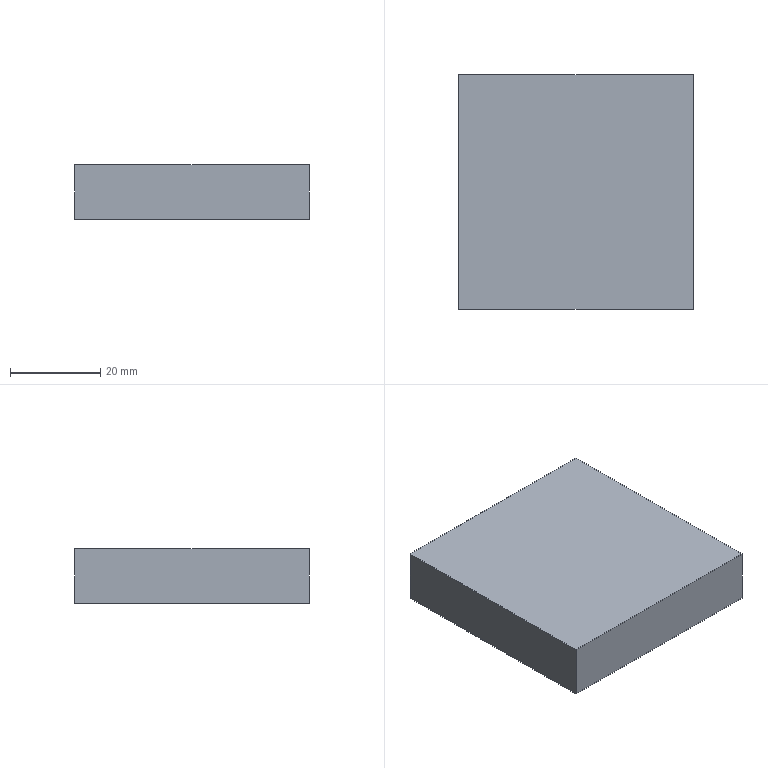NC program | NX | posted with a generic post | part box 52 x 52 x 12 mm
Whole program:
N10 G17 G21 G94 G90
(ADAPTIVE_MILLING_2 , TOOL : D4-12-D4-50-3T--FINISH)
N12 T02 M6
N14 G54
N16 G17 G0 G90 X33.202 Y5.386 S6500 M3
N18 G43 Z36. H2
N20 Z3.1
N22 G94 G1 X33.068 Y5.318 Z2.163 F2500.
N24 X32.934 Y5.251 Z1.792
N26 X32.8 Y5.184 Z1.52
N28 X32.666 Y5.117 Z1.3
N30 X32.532 Y5.05 Z1.116
N32 X32.398 Y4.982 Z0.958
N34 X32.263 Y4.915 Z0.82
N36 X32.129 Y4.848 Z0.7
N38 X31.995 Y4.781 Z0.595
N40 X31.861 Y4.713 Z0.502
N42 X31.727 Y4.646 Z0.421
N44 X31.593 Y4.579 Z0.35
N46 X31.459 Y4.512 Z0.29
N48 X31.325 Y4.445 Z0.238
N50 X31.191 Y4.377 Z0.195
N52 X31.057 Y4.31 Z0.161
N54 X30.923 Y4.243 Z0.134
N56 X30.788 Y4.176 Z0.115
N58 X30.654 Y4.108 Z0.104
N60 X30.52 Y4.041 Z0.1
N62 G3 X29.613 Y3.566 R20.387
N64 X29.267 Y2.553 R1.973
N66 X29.103 Y-1.691 R35.416
N68 G1 X29.1 Y-4.187
N70 Y-26.087
N72 G2 X27.654 Y-28.361 R2.481
N74 X24.899 Y-29.009 R6.987
N76 X18.651 Y-29.1 R108.628
N78 G1 X-26.099 Y-29.099
N80 G2 X-28.367 Y-27.643 R2.483
N82 X-29.01 Y-24.887 R7.02
N84 X-29.1 Y-18.639 R109.428
N86 G1 X-29.099 Y26.111
N88 G2 X-27.677 Y28.349 R2.466
N90 X-25.025 Y28.999 R6.751
N92 X-18.677 Y29.1 R98.255
N94 G1 X26.073 Y29.099
N96 G2 X28.355 Y27.665 R2.475
N98 X29.008 Y24.913 R6.92
N100 X29.1 Y18.614 R108.442
N102 G1 X29.098 Y4.814
N104 G2 X28.814 Y1.851 R288.734
N106 G3 X28.7 Y-4.537 R108.265
N108 G1 X28.699 Y-25.137
N110 G2 X26.921 Y-27.836 R3.109
N112 X23.884 Y-28.585 R7.808
N114 X18.587 Y-28.699 R76.943
N116 G1 X-24.987 Y-28.7
N118 G2 X-27.789 Y-27.009 R3.08
N120 X-28.576 Y-23.984 R7.492
N122 X-28.699 Y-18.437 R74.696
N124 G1 X-28.7 Y24.987
N126 G2 X-27.009 Y27.789 R3.077
N128 X-23.983 Y28.576 R7.502
N130 X-18.286 Y28.699 R76.887
N132 G1 X24.987 Y28.7
N134 G2 X27.836 Y26.922 R3.107
N136 X28.576 Y23.984 R7.67
N138 X28.699 Y18.287 R76.816
N140 G1 Y5.937
N142 G2 X28.446 Y2.154 R57.462
N144 G3 X28.3 Y-4.637 R109.004
N146 G1 X28.299 Y-24.137
N148 G2 X26.157 Y-27.429 R3.588
N150 X22.861 Y-28.186 R9.02
N152 X15.763 Y-28.3 R112.737
N154 G1 X-24.137 Y-28.299
N156 G2 X-27.429 Y-26.157 R3.586
N158 X-28.186 Y-22.861 R9.024
N160 X-28.3 Y-15.763 R112.852
N162 G1 X-28.299 Y24.137
N164 G2 X-26.157 Y27.429 R3.585
N166 X-22.96 Y28.178 R8.864
N168 X-16.013 Y28.299 R103.346
N170 G1 X24.137 Y28.298
N172 G2 X27.429 Y26.158 R3.589
N174 X28.178 Y22.961 R8.859
N176 X28.299 Y16.013 R103.354
N178 X28.274 Y5.514 R625.772
N180 G3 X27.946 Y-0.326 R181.868
N182 X27.9 Y-5.987 R563.769
N184 G1 X27.899 Y-23.237
N186 G2 X25.446 Y-27.038 R3.966
N188 X22.045 Y-27.782 R9.931
N190 X14.697 Y-27.899 R117.932
N192 G1 X-23.253 Y-27.898
N194 G2 X-27.018 Y-25.489 R3.952
N196 X-27.778 Y-22.093 R9.772
N198 X-27.899 Y-16.345 R87.299
N200 G1 Y23.055
N202 G2 X-26.901 Y26.005 R4.044
N204 X-23.951 Y27.523 R5.502
N206 X-19.622 Y27.879 R23.323
N208 G1 X-14.973 Y27.899
N210 X23.227 Y27.898
N212 G2 X27.037 Y25.446 R3.966
N214 X27.786 Y21.995 R10.006
N216 X27.899 Y14.998 R114.182
N218 X27.864 Y5.648 R387.941
N220 G3 X27.516 Y-2.353 R158.908
N222 G1 X27.501 Y-5.637
N224 X27.499 Y-22.387
N226 G2 X26.582 Y-25.33 R4.427
N228 X23.64 Y-27.033 R5.413
N230 X19.471 Y-27.464 R19.676
N232 X14.171 Y-27.499 R562.151
N234 G1 X-22.379 Y-27.498
N236 G2 X-25.206 Y-26.681 R4.473
N238 X-27.007 Y-23.737 R5.279
N240 X-27.464 Y-19.471 R19.146
N242 X-27.499 Y-14.171 R562.14
N244 G1 X-27.498 Y22.379
N246 G2 X-26.681 Y25.206 R4.473
N248 X-23.737 Y27.007 R5.27
N250 X-19.52 Y27.463 R18.996
N252 X-14.171 Y27.499 R562.312
N254 G1 X22.429 Y27.497
N256 G2 X25.587 Y26.352 R4.319
N258 X27.122 Y23.251 R5.907
N260 X27.478 Y18.772 R25.018
N262 X27.46 Y5.872 R471.898
N264 G3 X27.115 Y-2.751 R190.612
N266 G1 X27.1 Y-6.637
N268 X27.099 Y-21.637
N270 G2 X26.432 Y-24.418 R5.072
N272 X23.562 Y-26.475 R5.084
N274 X19.663 Y-27.032 R15.373
N276 X13.063 Y-27.099 R207.513
N278 G1 X-21.637 Y-27.097
N280 G2 X-24.417 Y-26.432 R5.072
N282 X-26.475 Y-23.562 R5.084
N284 X-27.032 Y-19.663 R15.375
N286 X-27.099 Y-13.063 R207.359
N288 G1 X-27.097 Y21.637
N290 G2 X-26.431 Y24.42 R5.069
N292 X-23.562 Y26.474 R5.086
N294 X-19.661 Y27.032 R15.384
N296 X-12.811 Y27.099 R214.459
N298 G1 X21.639 Y27.097
N300 G2 X24.419 Y26.43 R5.068
N302 X26.474 Y23.562 R5.084
N304 X27.038 Y19.513 R15.741
N306 X27.046 Y5.765 R329.265
N308 G3 X26.701 Y-6.587 R189.684
N310 G1 X26.699 Y-20.887
N312 G2 X26.176 Y-23.61 R5.851
N314 X23.287 Y-25.969 R5.
N316 X19.253 Y-26.618 R14.345
N318 X12.404 Y-26.699 R173.824
N320 G1 X-20.896 Y-26.697
N322 G2 X-23.662 Y-26.148 R5.788
N324 X-26.002 Y-23.192 R5.055
N326 X-26.618 Y-19.253 R14.659
N328 X-26.699 Y-12.404 R173.965
N330 G1 X-26.697 Y20.896
N332 G2 X-26.148 Y23.663 R5.789
N334 X-23.286 Y25.969 R5.01
N336 X-19.252 Y26.618 R14.365
N338 X-12.403 Y26.699 R173.957
N340 G1 X20.897 Y26.697
N342 G2 X23.662 Y26.147 R5.784
N344 X25.968 Y23.286 R5.011
N346 X26.618 Y19.253 R14.353
N348 X26.699 Y12.404 R173.976
N350 X26.42 Y1.202 R160.245
N352 G3 X26.301 Y-6.537 R225.077
N354 G1 X26.299 Y-20.237
N356 G2 X25.822 Y-22.973 R6.442
N358 X22.862 Y-25.519 R5.053
N360 X18.784 Y-26.208 R14.133
N362 X11.735 Y-26.299 R159.531
N364 G1 X-20.115 Y-26.298
N366 G2 X-22.815 Y-25.891 R6.94
N368 X-25.483 Y-22.956 R4.972
N370 X-26.191 Y-19.084 R13.197
N372 X-26.299 Y-11.686 R138.826
N374 G1 X-26.298 Y20.114
N376 G2 X-25.892 Y22.815 R6.943
N378 X-23.048 Y25.447 R4.933
N380 X-19.133 Y26.187 R12.861
N382 X-11.385 Y26.299 R142.121
N384 G1 X20.115 Y26.298
N386 G2 X22.816 Y25.891 R6.942
N388 X25.447 Y23.048 R4.934
N390 X26.187 Y19.133 R12.86
N392 X26.298 Y13.035 R113.031
N394 X26.017 Y1.056 R180.36
N396 G3 X25.901 Y-6.687 R244.494
N398 G1 X25.899 Y-19.537
N400 G2 X25.49 Y-22.289 R7.335
N402 X22.525 Y-25.042 R5.059
N404 X18.51 Y-25.788 R13.381
N406 X11.012 Y-25.898 R140.189
N408 G1 X-19.538 Y-25.897
N410 G2 X-22.29 Y-25.489 R7.319
N412 X-25.042 Y-22.525 R5.059
N414 X-25.788 Y-18.51 R13.38
N416 X-25.898 Y-11.012 R140.406
N418 G1 X-25.897 Y19.538
N420 G2 X-25.489 Y22.29 R7.319
N422 X-22.525 Y25.042 R5.058
N424 X-18.558 Y25.784 R13.271
N426 X-11.01 Y25.898 R136.948
N428 G1 X19.54 Y25.897
N430 G2 X22.292 Y25.489 R7.32
N432 X25.042 Y22.525 R5.057
N434 X25.784 Y18.558 R13.27
N436 X25.898 Y11.01 R136.967
N438 X25.629 Y1.304 R174.016
N440 G3 X25.501 Y-7.937 R255.072
N442 G2 X25.48 Y-19.687 R858.965
N444 X24.409 Y-22.953 R5.395
N446 X21.164 Y-24.916 R6.068
N448 X16.555 Y-25.449 R20.474
N450 X10.305 Y-25.498 R402.469
N452 G1 X-18.945 Y-25.496
N454 G2 X-21.75 Y-25.098 R7.77
N456 X-24.606 Y-22.093 R5.14
N458 X-25.377 Y-18.08 R13.247
N460 X-25.498 Y-10.232 R136.021
N462 G1 X-25.496 Y18.918
N464 G2 X-25.089 Y21.771 R7.792
N466 X-22.158 Y24.58 R5.111
N468 X-18.252 Y25.365 R12.781
N470 X-11.855 Y25.497 R101.053
N472 G1 X18.595 Y25.498
N474 G2 X21.42 Y25.213 R9.68
N476 X24.534 Y22.265 R5.026
N478 X25.36 Y18.315 R12.384
N480 X25.498 Y10.818 R114.882
N482 X25.224 Y1.108 R198.056
N484 G3 X25.101 Y-8.137 R275.31
N486 G2 X25.077 Y-19.187 R738.948
N488 X24.01 Y-22.469 R5.522
N490 X20.732 Y-24.491 R6.115
N492 X16.125 Y-25.044 R20.119
N494 X9.525 Y-25.098 R336.072
N496 G1 X-18.275 Y-25.096
N498 G2 X-21.091 Y-24.753 R8.79
N500 X-24.156 Y-21.71 R5.166
N502 X-24.971 Y-17.608 R13.131
N504 X-25.098 Y-9.51 R136.193
N506 G1 X-25.097 Y18.24
N508 G2 X-24.748 Y21.105 R8.853
N510 X-21.679 Y24.168 R5.182
N512 X-17.772 Y24.958 R12.929
N514 X-11.175 Y25.097 R100.428
N516 G1 X17.975 Y25.098
N518 G2 X20.852 Y24.828 R10.533
N520 X24.155 Y21.709 R5.134
N522 X24.97 Y17.608 R13.125
N524 X25.085 Y8.56 R140.756
N526 X24.781 Y-0.328 R617.832
N528 G3 X24.701 Y-7.987 R409.354
N530 G2 X24.679 Y-18.587 R582.556
N532 X23.748 Y-21.807 R5.887
N534 X20.499 Y-24.011 R5.943
N536 X16.053 Y-24.625 R18.072
N538 X9.354 Y-24.698 R214.25
N540 G1 X-17.746 Y-24.696
N542 G2 X-20.659 Y-24.329 R8.921
N544 X-23.737 Y-21.26 R5.247
N546 X-24.559 Y-17.209 R13.059
N548 X-24.698 Y-9.262 R124.319
N550 G1 X-24.697 Y17.638
N552 G2 X-24.364 Y20.557 R9.509
N554 X-21.292 Y23.722 R5.218
N556 X-17.245 Y24.556 R12.962
N558 X-9.297 Y24.698 R122.564
N560 G1 X17.453 Y24.697
N562 G2 X20.331 Y24.432 R10.914
N564 X23.697 Y21.351 R5.174
N566 X24.552 Y17.306 R12.707
N568 X24.686 Y8.859 R116.175
N570 X24.379 Y-0.476 R641.834
N572 G3 X24.3 Y-17.037 R774.98
N574 G2 X23.998 Y-19.961 R10.483
N576 X20.839 Y-23.31 R5.278
N578 X16.842 Y-24.146 R12.943
N580 X10.145 Y-24.297 R96.908
N582 G1 X-16.805
N584 G2 X-19.834 Y-24.032 R11.774
N586 X-23.281 Y-20.906 R5.246
N588 X-24.14 Y-16.916 R12.628
N590 X-24.297 Y-10.169 R94.338
N592 G1 X-24.298 Y16.831
N594 G2 X-24.039 Y19.811 R11.87
N596 X-20.931 Y23.269 R5.236
N598 X-16.842 Y24.146 R12.728
N600 X-10.096 Y24.297 R97.143
N602 G1 X16.754
N604 G2 X19.737 Y24.058 R12.501
N606 X23.28 Y20.905 R5.239
N608 X24.14 Y16.915 R12.643
N610 X24.268 Y7.969 R106.869
N612 X23.983 Y-0.426 R862.542
N614 G3 X23.898 Y-16.687 R753.99
N616 G2 X23.527 Y-19.701 R9.605
N618 X20.418 Y-22.885 R5.359
N620 X16.324 Y-23.746 R13.053
N622 X9.377 Y-23.897 R101.419
N624 G1 X-15.723 Y-23.898
N626 G2 X-19.012 Y-23.711 R17.095
N628 X-22.846 Y-20.509 R5.286
N630 X-23.729 Y-16.523 R12.506
N632 X-23.897 Y-9.327 R95.572
N634 G1 X-23.898 Y15.773
N636 G2 X-23.711 Y19.012 R16.787
N638 X-20.51 Y22.844 R5.283
N640 X-16.424 Y23.737 R12.688
N642 X-9.778 Y23.896 R92.352
N644 G1 X16.222 Y23.897
N646 G2 X19.352 Y23.631 R12.491
N648 X22.885 Y20.418 R5.325
N650 X23.749 Y16.272 R13.169
N652 X23.782 Y5.076 R114.009
N654 G3 X23.501 Y-8.937 R282.906
N656 G2 X23.468 Y-17.236 R320.538
N658 X22.465 Y-20.539 R6.073
N660 X19.104 Y-22.79 R6.197
N662 X14.708 Y-23.413 R18.283
N664 X7.459 Y-23.497 R194.607
N666 G1 X-15.991 Y-23.496
N668 G2 X-19.015 Y-23.191 R11.169
N670 X-22.465 Y-19.995 R5.393
N672 X-23.338 Y-15.906 R13.031
N674 X-23.496 Y-9.059 R96.326
N676 G1 X-23.497 Y15.691
N678 G2 X-23.256 Y18.774 R13.391
N680 X-19.995 Y22.464 R5.376
N682 X-15.806 Y23.345 R13.22
N684 X-9.06 Y23.496 R99.201
N686 G1 X15.64 Y23.497
N688 G2 X18.774 Y23.256 R13.595
N690 X22.464 Y19.995 R5.377
N692 X23.333 Y15.956 R12.973
N694 X23.422 Y6.36 R97.927
N696 G3 X23.102 Y-8.337 R336.38
N698 G2 X23.067 Y-16.736 R327.372
N700 X22.063 Y-20.091 R6.211
N702 X18.733 Y-22.359 R6.207
N704 X14.393 Y-23.003 R17.732
N706 X6.644 Y-23.097 R185.5
N708 G1 X-15.156
N710 G2 X-18.387 Y-22.834 R13.491
N712 X-22.04 Y-19.589 R5.426
N714 X-22.938 Y-15.403 R13.138
N716 X-23.096 Y-8.757 R94.642
N718 G1 X-23.097 Y14.593
N720 G2 X-22.924 Y17.984 R19.339
N722 X-19.524 Y22.067 R5.433
N724 X-15.28 Y22.947 R13.527
N726 X-8.783 Y23.096 R97.673
N728 G1 X15.117 Y23.097
N730 G2 X18.3 Y22.855 R14.063
N732 X22.059 Y19.542 R5.435
N734 X22.945 Y15.302 R13.45
N736 X22.992 Y5.506 R99.559
N738 G3 X22.701 Y-9.237 R311.474
N740 G2 X22.668 Y-16.236 R221.924
N742 X21.72 Y-19.56 R6.414
N744 X18.366 Y-21.927 R6.181
N746 X13.778 Y-22.608 R18.
N748 X6.379 Y-22.697 R190.758
N750 G1 X-14.621
N752 G2 X-17.854 Y-22.451 R14.365
N754 X-21.666 Y-19.069 R5.499
N756 X-22.528 Y-15.026 R13.282
N758 X-22.696 Y-7.93 R96.097
N760 G1 X-22.697 Y14.62
N762 G2 X-22.45 Y17.853 R14.292
N764 X-19.069 Y21.665 R5.496
N766 X-14.926 Y22.536 R13.472
N768 X-7.93 Y22.696 R98.754
N770 G1 X14.57 Y22.697
N772 G2 X17.853 Y22.45 R14.565
N774 X21.665 Y19.069 R5.496
N776 X22.527 Y15.026 R13.304
N778 X22.598 Y5.781 R89.279
N780 G3 X22.302 Y-8.887 R332.008
N782 G2 X22.257 Y-15.936 R187.741
N784 X21.117 Y-19.402 R6.15
N786 X17.722 Y-21.584 R6.471
N788 X13.077 Y-22.218 R19.505
N790 X5.578 Y-22.297 R221.492
N792 G1 X-14.422 Y-22.295
N794 G2 X-17.647 Y-21.983 R12.204
N796 X-21.225 Y-18.709 R5.531
N798 X-22.133 Y-14.475 R13.337
N800 X-22.296 Y-7.629 R96.425
N802 G1 X-22.297 Y14.071
N804 G2 X-22.047 Y17.404 R14.798
N806 X-18.709 Y21.224 R5.519
N808 X-14.623 Y22.12 R13.119
N810 X-7.628 Y22.296 R91.875
N812 G1 X13.522 Y22.297
N814 G2 X17.063 Y22.119 R20.553
N816 X21.224 Y18.709 R5.521
N818 X22.12 Y14.624 R13.108
N820 X22.201 Y5.978 R82.174
N822 G3 X21.9 Y-13.787 R430.309
N824 G2 X21.62 Y-17.066 R13.646
N826 X18.242 Y-20.833 R5.587
N828 X14.005 Y-21.732 R13.549
N830 X6.959 Y-21.896 R99.113
N832 G1 X-12.991 Y-21.897
N834 G2 X-16.533 Y-21.731 R22.03
N836 X-20.816 Y-18.281 R5.567
N838 X-21.721 Y-14.145 R13.212
N840 X-21.896 Y-6.799 R96.828
N842 G1 X-21.897 Y13.551
N844 G2 X-21.671 Y16.837 R16.007
N846 X-18.274 Y20.819 R5.564
N848 X-14.038 Y21.729 R13.479
N850 X-6.792 Y21.896 R99.839
N852 G1 X13.508 Y21.897
N854 G2 X16.844 Y21.67 R16.225
N856 X20.83 Y18.245 R5.573
N858 X21.723 Y14.107 R13.349
N860 X21.791 Y5.711 R80.555
N862 G3 X21.498 Y-13.637 R436.187
N864 G2 X21.152 Y-16.858 R11.661
N866 X17.819 Y-20.425 R5.641
N868 X13.683 Y-21.32 R13.456
N870 X6.687 Y-21.495 R92.893
N872 G1 X-13.013 Y-21.496
N874 G2 X-16.448 Y-21.257 R16.2
N876 X-20.436 Y-17.788 R5.623
N878 X-21.322 Y-13.65 R13.527
N880 X-21.496 Y-6.504 R95.873
N882 G1 Y12.996
N884 G2 X-21.271 Y16.382 R16.682
N886 X-17.789 Y20.435 R5.624
N888 X-13.65 Y21.322 R13.523
N890 X-6.504 Y21.495 R95.469
N892 G1 X12.446 Y21.497
N894 G2 X16.087 Y21.329 R22.766
N896 X20.435 Y17.788 R5.628
N898 X21.336 Y13.45 R13.828
N900 X21.361 Y4.854 R85.654
N902 G3 X21.095 Y-13.387 R445.794
N904 G2 X20.709 Y-16.551 R10.716
N906 X17.431 Y-20. R5.665
N908 X13.147 Y-20.925 R13.549
N910 X5.851 Y-21.096 R99.974
N912 G1 X-12.449
N914 G2 X-15.935 Y-20.87 R17.378
N916 X-20.024 Y-17.374 R5.654
N918 X-20.93 Y-13.085 R13.806
N920 X-21.095 Y-6.239 R96.548
N922 G1 X-21.096 Y12.461
N924 G2 X-20.878 Y15.898 R17.582
N926 X-17.364 Y20.028 R5.657
N928 X-13.076 Y20.93 R13.885
N930 X-6.229 Y21.095 R96.926
N932 G1 X12.471 Y21.096
N934 G2 X15.957 Y20.865 R17.079
N936 X19.989 Y17.453 R5.631
N938 X20.911 Y13.27 R13.256
N940 X20.967 Y5.125 R76.421
N942 G3 X20.691 Y-13.137 R470.026
N944 G2 X20.23 Y-16.338 R9.725
N946 X16.917 Y-19.633 R5.748
N948 X12.577 Y-20.533 R14.073
N950 X5.581 Y-20.695 R101.382
N952 G1 X-11.969 Y-20.696
N954 G2 X-15.407 Y-20.487 R18.345
N956 X-19.605 Y-16.977 R5.687
N958 X-20.507 Y-12.891 R13.336
N960 X-20.695 Y-5.345 R94.863
N962 G1 X-20.696 Y11.955
N964 G2 X-20.479 Y15.442 R18.124
N966 X-16.906 Y19.635 R5.704
N968 X-12.667 Y20.526 R13.991
N970 X-5.37 Y20.695 R101.003
N972 G1 X11.98 Y20.696
N974 G2 X15.466 Y20.474 R17.815
N976 X19.587 Y17.016 R5.667
N978 X20.502 Y12.884 R13.17
N980 X20.571 Y5.338 R70.719
N982 G3 X20.289 Y-12.787 R490.925
N984 G2 X19.799 Y-15.983 R9.441
N986 X16.46 Y-19.242 R5.806
N988 X12.118 Y-20.133 R14.284
N990 X4.772 Y-20.295 R106.716
N992 G1 X-11.478 Y-20.296
N994 G2 X-15.015 Y-20.076 R18.362
N996 X-19.201 Y-16.552 R5.716
N998 X-20.125 Y-12.219 R13.86
N1000 X-20.295 Y-5.023 R100.054
N1002 G1 X-20.296 Y11.477
N1004 G2 X-20.076 Y15.014 R18.361
N1006 X-16.553 Y19.2 R5.712
N1008 X-12.269 Y20.12 R13.789
N1010 X-5.023 Y20.295 R98.293
N1012 G1 X11.477 Y20.296
N1014 G2 X15.014 Y20.076 R18.397
N1016 X19.22 Y16.502 R5.726
N1018 X20.119 Y12.163 R13.88
N1020 X20.143 Y4.467 R78.566
N1022 G3 X19.891 Y-12.237 R456.053
N1024 G2 X19.405 Y-15.535 R9.81
N1026 X15.995 Y-18.854 R5.85
N1028 X11.598 Y-19.738 R14.639
N1030 X4.701 Y-19.895 R104.179
N1032 G1 X-10.949 Y-19.896
N1034 G2 X-14.488 Y-19.693 R19.795
N1036 X-18.807 Y-16.102 R5.76
N1038 X-19.725 Y-11.767 R13.991
N1040 X-19.895 Y-4.721 R98.377
N1042 G1 X-19.896 Y10.979
N1044 G2 X-19.687 Y14.518 R19.289
N1046 X-16.092 Y18.812 R5.756
N1048 X-11.755 Y19.725 R14.105
N1050 X-4.708 Y19.895 R98.478
N1052 G1 X10.942 Y19.896
N1054 G2 X14.53 Y19.685 R19.465
N1056 X18.817 Y16.076 R5.762
N1058 X19.713 Y11.735 R13.893
N1060 X19.732 Y4.188 R77.923
N1062 G3 X19.486 Y-11.988 R511.045
N1064 G2 X18.957 Y-15.227 R9.201
N1066 X15.554 Y-18.457 R5.894
N1068 X11.159 Y-19.337 R14.71
N1070 X4.263 Y-19.494 R104.098
N1072 G1 X-10.437 Y-19.496
N1074 G2 X-14.076 Y-19.288 R20.039
N1076 X-18.356 Y-15.788 R5.752
N1078 X-19.304 Y-11.559 R13.432
N1080 X-19.495 Y-3.864 R96.856
N1082 G1 X-19.496 Y10.436
N1084 G2 X-19.287 Y14.075 R20.059
N1086 X-15.787 Y18.356 R5.746
N1088 X-11.558 Y19.303 R13.465
N1090 X-4.412 Y19.494 R89.82
N1092 G1 X10.438 Y19.496
N1094 G2 X14.076 Y19.288 R20.066
N1096 X18.355 Y15.786 R5.744
N1098 X19.298 Y11.405 R13.414
N1100 X19.337 Y4.408 R71.948
N1102 G3 X19.088 Y-11.438 R481.811
N1104 G2 X18.601 Y-14.686 R9.808
N1106 X15.188 Y-18.031 R5.882
N1108 X10.897 Y-18.922 R14.36
N1110 X3.601 Y-19.094 R101.293
N1112 G1 X-9.949 Y-19.096
N1114 G2 X-13.589 Y-18.897 R21.022
N1116 X-17.973 Y-15.323 R5.795
N1118 X-18.906 Y-11.091 R13.687
N1120 X-19.095 Y-3.546 R96.363
N1122 G1 X-19.096 Y10.004
N1124 G2 X-18.887 Y13.643 R20.229
N1126 X-15.32 Y17.973 R5.79
N1128 X-11.14 Y18.901 R13.631
N1130 X-3.495 Y19.095 R95.28
N1132 G1 X9.955
N1134 G2 X13.644 Y18.887 R20.482
N1136 X17.972 Y15.317 R5.783
N1138 X18.894 Y10.931 R13.634
N1140 X18.925 Y4.084 R72.837
N1142 G3 X18.683 Y-11.189 R550.02
N1144 G2 X18.117 Y-14.471 R9.057
N1146 X14.737 Y-17.64 R5.951
N1148 X10.442 Y-18.523 R14.501
N1150 X3.345 Y-18.694 R99.146
N1152 G1 X-9.505 Y-18.695
N1154 G2 X-13.194 Y-18.49 R20.903
N1156 X-17.568 Y-14.908 R5.818
N1158 X-18.516 Y-10.529 R13.94
N1160 X-18.694 Y-3.183 R99.112
N1162 G1 X-18.695 Y9.517
N1164 G2 X-18.496 Y13.157 R21.189
N1166 X-14.84 Y17.595 R5.829
N1168 X-10.555 Y18.513 R14.074
N1170 X-3.26 Y18.694 R96.807
N1172 G1 X9.49 Y18.695
N1174 G2 X13.18 Y18.493 R21.158
N1176 X17.581 Y14.866 R5.813
N1178 X18.488 Y10.477 R13.758
N1180 X18.513 Y3.73 R73.804
N1182 G3 X18.28 Y-10.84 R603.062
N1184 G2 X17.666 Y-14.163 R8.758
N1186 X14.234 Y-17.272 R6.025
N1188 X9.734 Y-18.143 R15.352
N1190 X1.187 Y-18.295 R136.707
N1192 X-11.013 Y-18.268 R817.727
N1194 X-14.321 Y-17.588 R8.209
N1196 X-17.266 Y-14.245 R6.051
N1198 X-18.142 Y-9.746 R15.244
N1200 X-18.295 Y-1.199 R136.008
N1202 X-18.266 Y11.05 R740.37
N1204 X-17.55 Y14.398 R8.042
N1206 X-14.165 Y17.296 R6.099
N1208 X-9.61 Y18.151 R15.764
N1210 X-1.063 Y18.295 R142.458
N1212 X10.987 Y18.269 R840.51
N1214 X14.25 Y17.621 R8.352
N1216 X17.285 Y14.177 R6.023
N1218 X18.1 Y9.718 R14.964
N1220 X18.103 Y3.419 R80.665
N1222 G3 X17.884 Y-10.291 R552.078
N1224 G2 X17.317 Y-13.623 R9.281
N1226 X13.962 Y-16.811 R5.969
N1228 X9.623 Y-17.718 R14.443
N1230 X2.327 Y-17.894 R100.074
N1232 X-10.473 Y-17.871 R887.942
N1234 X-13.745 Y-17.26 R8.687
N1236 X-16.866 Y-13.823 R6.049
N1238 X-17.741 Y-9.324 R15.315
N1240 X-17.895 Y-0.828 R133.093
N1242 X-17.863 Y10.672 R601.608
N1244 X-17.13 Y14.015 R7.95
N1246 X-13.788 Y16.877 R6.117
N1248 X-9.387 Y17.736 R15.302
N1250 X-2.541 Y17.893 R104.146
N1252 X10.459 Y17.871 R899.943
N1254 X13.732 Y17.265 R8.744
N1256 X16.855 Y13.821 R6.
N1258 X17.689 Y9.316 R14.741
N1260 X17.69 Y3.018 R81.56
N1262 G3 X17.484 Y-9.891 R592.296
N1264 G2 X16.909 Y-13.222 R9.253
N1266 X13.449 Y-16.447 R6.026
N1268 X8.952 Y-17.336 R15.179
N1270 X0.555 Y-17.495 R128.066
N1272 X-10.295 Y-17.461 R501.495
N1274 X-13.589 Y-16.734 R7.954
N1276 X-16.524 Y-13.245 R6.181
N1278 X-17.358 Y-8.635 R16.328
N1280 X-17.495 Y-0.488 R142.529
N1282 X-17.468 Y10.112 R591.914
N1284 X-16.791 Y13.47 R8.398
N1286 X-13.328 Y16.493 R6.117
N1288 X-8.822 Y17.345 R15.773
N1290 X-1.625 Y17.494 R115.961
N1292 X10.224 Y17.463 R635.338
N1294 X13.526 Y16.765 R8.132
N1296 X16.503 Y13.266 R6.109
N1298 X17.281 Y8.848 R15.202
N1300 X17.264 Y2.099 R89.763
N1302 G3 X17.083 Y-9.493 R666.233
N1304 G2 X16.5 Y-12.823 R9.204
N1306 X13.029 Y-16.046 R6.054
N1308 X8.534 Y-16.935 R15.213
N1310 X1.237 Y-17.094 R110.95
N1312 X-9.662 Y-17.068 R724.519
N1314 X-12.978 Y-16.426 R8.608
N1316 X-16.049 Y-13.018 R6.076
N1318 X-16.92 Y-8.722 R14.872
N1320 X-17.094 Y-1.276 R104.132
N1322 X-17.062 Y9.824 R549.887
N1324 X-16.334 Y13.169 R8.063
N1326 X-12.912 Y16.091 R6.163
N1328 X-8.408 Y16.943 R15.804
N1330 X-1.211 Y17.094 R115.606
N1332 X9.838 Y17.061 R527.663
N1334 X13.137 Y16.35 R8.066
N1336 X16.085 Y12.883 R6.119
N1338 X16.879 Y8.269 R15.445
N1340 X16.819 Y0.376 R117.397
N1342 G3 X16.685 Y-9.044 R733.253
N1344 G2 X16.112 Y-12.377 R9.35
N1346 X12.715 Y-15.603 R6.025
N1348 X8.325 Y-16.517 R14.599
N1350 X0.928 Y-16.694 R102.307
N1352 X-9.471 Y-16.658 R435.207
N1354 X-12.809 Y-15.905 R7.928
N1356 X-15.726 Y-12.399 R6.238
N1358 X-16.55 Y-7.888 R16.267
N1360 X-16.695 Y0.759 R144.688
N1362 X-16.656 Y9.509 R334.077
N1364 X-15.863 Y12.887 R7.77
N1366 X-12.42 Y15.718 R6.25
N1368 X-7.911 Y16.548 R16.214
N1370 X0.787 Y16.695 R144.214
N1372 X9.586 Y16.652 R296.219
N1374 X13.001 Y15.8 R7.543
N1376 X15.718 Y12.357 R6.239
N1378 X16.472 Y7.735 R15.945
N1380 X16.419 Y0.376 R117.826
N1382 G3 X16.285 Y-8.646 R739.371
N1384 G2 X15.706 Y-11.976 R9.324
N1386 X12.251 Y-15.223 R6.062
N1388 X7.76 Y-16.128 R15.036
N1390 X0.363 Y-16.294 R108.953
N1392 X-8.936 Y-16.263 R425.598
N1394 X-12.332 Y-15.536 R8.219
N1396 X-15.293 Y-12.067 R6.203
N1398 X-16.149 Y-7.463 R16.118
N1400 X-16.295 Y1.085 R143.313
N1402 X-16.251 Y9.184 R253.955
N1404 X-15.394 Y12.597 R7.541
N1406 X-11.88 Y15.362 R6.357
N1408 X-7.263 Y16.162 R17.111
N1410 X1.185 Y16.294 R154.351
N1412 X9.184 Y16.25 R250.688
N1414 X12.594 Y15.394 R7.525
N1416 X15.327 Y11.897 R6.277
N1418 X16.061 Y7.321 R16.114
N1420 X15.996 Y-0.62 R132.737
N1422 X15.863 Y-8.746 R739.383
N1424 X15.037 Y-12.118 R7.712
N1426 X11.574 Y-14.924 R6.313
N1428 X7.063 Y-15.747 R16.359
N1430 X-1.334 Y-15.894 R139.212
N1432 X-8.734 Y-15.852 R234.719
N1434 X-12.106 Y-15.037 R7.691
N1436 X-14.907 Y-11.616 R6.278
N1438 X-15.754 Y-6.959 R16.459
N1440 X-15.894 Y1.539 R146.981
N1442 X-15.846 Y8.838 R197.948
N1444 X-14.935 Y12.284 R7.393
N1446 X-11.428 Y14.975 R6.418
N1448 X-6.809 Y15.764 R17.362
N1450 X1.489 Y15.894 R153.621
N1452 X8.788 Y15.849 R214.88
N1454 X12.154 Y15.007 R7.531
N1456 X14.914 Y11.498 R6.261
N1458 X15.65 Y6.871 R16.186
N1460 X15.6 Y-0.47 R127.114
N1462 X15.464 Y-8.348 R613.769
N1464 X14.607 Y-11.76 R7.662
N1466 X11.144 Y-14.528 R6.349
N1468 X6.583 Y-15.351 R16.539
N1470 X-1.915 Y-15.494 R144.582
N1472 X-8.464 Y-15.443 R162.143
N1474 X-11.904 Y-14.516 R7.345
N1476 X-14.581 Y-10.991 R6.464
N1478 X-15.364 Y-6.371 R17.487
N1480 X-15.494 Y1.927 R155.064
N1482 X-15.442 Y8.476 R159.595
N1484 X-14.508 Y11.915 R7.308
N1486 X-10.991 Y14.581 R6.463
N1488 X-6.371 Y15.364 R17.494
N1490 X1.877 Y15.494 R153.706
N1492 X8.526 Y15.439 R152.989
N1494 X12. Y14.449 R7.122
N1496 X14.551 Y10.955 R6.416
N1498 X15.246 Y6.272 R17.02
N1500 X15.18 Y-1.416 R151.386
N1502 X15.058 Y-8.049 R275.919
N1504 X14.125 Y-11.491 R7.41
N1506 X10.651 Y-14.157 R6.454
N1508 X6.085 Y-14.956 R17.048
N1510 X-2.313 Y-15.094 R148.323
N1512 X-8.162 Y-15.035 R110.375
N1514 X-11.673 Y-14.001 R7.073
N1516 X-14.212 Y-10.484 R6.596
N1518 X-14.972 Y-5.81 R18.148
N1520 X-15.094 Y2.288 R160.71
N1522 X-15.033 Y8.187 R117.285
N1524 X-14.015 Y11.651 R7.076
N1526 X-10.523 Y14.2 R6.564
N1528 X-5.85 Y14.97 R17.955
N1530 X2.248 Y15.094 R157.941
N1532 X8.097 Y15.039 R119.61
N1534 X11.571 Y14.057 R7.16
N1536 X14.149 Y10.522 R6.414
N1538 X14.837 Y5.787 R17.259
N1540 X14.765 Y-2.262 R171.254
N1542 X14.648 Y-7.8 R138.48
N1544 X13.613 Y-11.258 R7.1
N1546 X10.07 Y-13.815 R6.625
N1548 X5.295 Y-14.578 R18.502
N1550 X-2.804 Y-14.694 R168.663
N1552 X-8.051 Y-14.61 R73.459
N1554 X-11.71 Y-13.274 R6.526
N1556 X-13.914 Y-9.749 R7.02
N1558 X-14.597 Y-4.908 R20.54
N1560 X-14.655 Y7.39 R248.618
N1562 X-13.885 Y10.775 R8.031
N1564 X-10.341 Y13.716 R6.305
N1566 X-5.879 Y14.54 R16.31
N1568 X2.618 Y14.694 R136.036
N1570 X8.016 Y14.613 R78.902
N1572 X11.633 Y13.319 R6.524
N1574 X13.847 Y9.763 R6.83
N1576 X14.436 Y5.011 R19.311
N1578 X14.35 Y-3.208 R245.457
N1580 X14.212 Y-7.8 R59.501
N1582 X12.544 Y-11.682 R6.308
N1584 X8.931 Y-13.629 R7.57
N1586 X3.776 Y-14.227 R24.424
N1588 X-7.123 Y-14.247 R215.546
N1590 X-10.537 Y-13.392 R7.662
N1592 X-13.329 Y-9.89 R6.388
N1594 X-14.156 Y-5.229 R16.943
N1596 X-14.294 Y2.919 R144.143
N1598 X-14.197 Y7.766 R57.47
N1600 X-12.632 Y11.58 R6.335
N1602 X-8.959 Y13.619 R7.446
N1604 X-3.954 Y14.219 R23.759
N1606 X7.145 Y14.245 R208.543
N1608 X10.551 Y13.373 R7.536
N1610 X13.299 Y9.796 R6.316
N1612 X14.006 Y5.164 R16.674
N1614 X13.959 Y-2.66 R160.932
N1616 X13.812 Y-7.402 R61.365
N1618 X12.108 Y-11.313 R6.306
N1620 X8.387 Y-13.262 R7.718
N1622 X3.328 Y-13.827 R25.262
N1624 X-6.821 Y-13.839 R176.193
N1626 X-10.305 Y-12.887 R7.368
N1628 X-12.97 Y-9.364 R6.519
N1630 X-13.759 Y-4.746 R17.484
N1632 X-13.893 Y4.452 R169.022
N1634 X-13.676 Y8.191 R21.386
N1636 X-9.977 Y12.731 R5.996
N1638 X-5.649 Y13.69 R14.09
N1640 X2.046 Y13.892 R95.545
N1642 X7.244 Y13.806 R68.641
N1644 X10.887 Y12.451 R6.437
N1646 X13.053 Y8.854 R6.932
N1648 X13.619 Y3.899 R20.511
N1650 X13.467 Y-6.406 R255.357
N1652 X12.506 Y-9.889 R7.493
N1654 X8.935 Y-12.579 R6.55
N1656 X4.365 Y-13.357 R17.56
N1658 X-6.432 Y-13.437 R143.027
N1660 X-9.914 Y-12.477 R7.353
N1662 X-12.562 Y-8.974 R6.526
N1664 X-13.364 Y-4.256 R17.632
N1666 X-13.443 Y6.341 R151.07
N1668 X-12.524 Y9.836 R7.549
N1670 X-8.974 Y12.561 R6.493
N1672 X-4.406 Y13.354 R17.297
N1674 X6.341 Y13.442 R146.252
N1676 X9.701 Y12.585 R7.528
N1678 X12.413 Y9.169 R6.229
N1680 X13.172 Y4.599 R15.691
N1682 X13.151 Y-3.208 R143.903
N1684 X12.939 Y-7.149 R28.023
N1686 X9.041 Y-11.983 R6.091
N1688 X4.554 Y-12.914 R14.965
N1690 X-3.542 Y-13.092 R112.073
N1692 X-7.38 Y-12.873 R21.818
N1694 X-11.918 Y-9.181 R6.004
N1696 X-12.896 Y-4.755 R14.214
N1698 X-13.092 Y3.29 R102.595
N1700 X-12.9 Y7.231 R24.755
N1702 X-9.181 Y11.918 R6.009
N1704 X-4.805 Y12.891 R14.135
N1706 X3.04 Y13.092 R97.936
N1708 X7.132 Y12.914 R27.402
N1710 X11.885 Y9.073 R5.932
N1712 X12.737 Y4.622 R14.232
N1714 X12.759 Y-2.71 R107.316
N1716 X12.54 Y-6.75 R28.636
N1718 X8.772 Y-11.524 R6.067
N1720 X4.346 Y-12.496 R14.31
N1722 X-5.748 Y-12.626 R97.577
N1724 X-9.294 Y-11.548 R7.069
N1726 X-11.789 Y-8.072 R6.657
N1728 X-12.567 Y-3.349 R18.141
N1730 X-12.636 Y5.598 R111.041
N1732 X-11.71 Y9.041 R7.44
N1734 X-8.213 Y11.739 R6.485
N1736 X-3.598 Y12.552 R17.168
N1738 X5.599 Y12.636 R108.812
N1740 X9.079 Y11.662 R7.231
N1742 X11.649 Y8.197 R6.372
N1744 X12.361 Y3.515 R16.842
N1746 X12.266 Y-5.332 R121.205
N1748 X11.176 Y-8.876 R7.196
N1750 X7.564 Y-11.428 R6.746
N1752 X2.786 Y-12.177 R18.955
N1754 X-5.262 Y-12.231 R93.657
N1756 X-8.736 Y-11.246 R7.28
N1758 X-11.382 Y-7.682 R6.591
N1760 X-12.157 Y-3.11 R17.736
N1762 X-12.218 Y5.436 R85.06
N1764 X-11.033 Y9.052 R6.862
N1766 X-7.522 Y11.436 R6.826
N1768 X-2.792 Y12.175 R18.997
N1770 X5.255 Y12.23 R92.434
N1772 X8.684 Y11.249 R7.137
N1774 X11.263 Y7.719 R6.415
N1776 X11.955 Y2.984 R17.416
N1778 X11.857 Y-5.063 R93.994
N1780 X10.642 Y-8.664 R6.937
N1782 X6.985 Y-11.081 R6.948
N1784 X2.098 Y-11.791 R20.304
N1786 X-4.999 Y-11.818 R74.918
N1788 X-8.578 Y-10.68 R6.946
N1790 X-11.02 Y-7.162 R6.781
N1792 X-11.766 Y-2.535 R18.471
N1794 X-11.814 Y5.061 R72.787
N1796 X-10.614 Y8.669 R6.813
N1798 X-7.046 Y11.056 R6.877
N1800 X-2.313 Y11.779 R19.449
N1802 X5.083 Y11.81 R70.716
N1804 X8.711 Y10.539 R6.593
N1806 X10.949 Y7. R6.789
N1808 X11.557 Y2.201 R19.375
N1810 X11.447 Y-4.795 R72.86
N1812 X10.035 Y-8.524 R6.664
N1814 X6.452 Y-10.718 R7.183
N1816 X1.56 Y-11.397 R21.091
N1818 X-4.737 Y-11.404 R59.205
N1820 X-8.448 Y-10.071 R6.646
N1822 X-10.722 Y-6.425 R7.117
N1824 X-11.395 Y-1.583 R21.078
N1826 X-11.402 Y4.764 R58.527
N1828 X-10.026 Y8.505 R6.599
N1830 X-6.445 Y10.714 R7.134
N1832 X-1.503 Y11.398 R21.172
N1834 X4.744 Y11.401 R57.701
N1836 X8.394 Y10.062 R6.468
N1838 X10.585 Y6.431 R6.946
N1840 X11.154 Y1.576 R20.652
N1842 X11.047 Y-4.421 R59.428
N1844 X9.613 Y-8.147 R6.637
N1846 X5.925 Y-10.354 R7.283
N1848 X0.828 Y-11.01 R22.566
N1850 X-4.518 Y-10.983 R44.675
N1852 X-8.415 Y-9.345 R6.349
N1854 X-10.422 Y-5.651 R7.605
N1856 X-11.019 Y-0.596 R24.372
N1858 X-10.975 Y4.601 R42.073
N1860 X-9.171 Y8.591 R6.243
N1862 X-5.457 Y10.47 R7.923
N1864 X-0.146 Y11.034 R26.78
N1866 X4.699 Y10.959 R36.614
N1868 X9.16 Y8.345 R5.925
N1870 X10.512 Y4.353 R9.632
N1872 X10.758 Y-1.737 R42.55
N1874 X10.404 Y-5.411 R15.628
N1876 X6.724 Y-9.53 R6.101
N1878 X2.247 Y-10.499 R14.578
N1880 X-4.196 Y-10.57 R40.628
N1882 X-8.205 Y-8.75 R6.232
N1884 X-10.073 Y-5.041 R7.96
N1886 X-10.63 Y0.171 R26.459
N1888 X-10.524 Y4.564 R27.948
N1890 X-6.719 Y9.522 R6.069
N1892 X-2.193 Y10.501 R14.575
N1894 X4.15 Y10.571 R40.195
N1896 X8.146 Y8.715 R6.081
N1898 X9.914 Y5.009 R7.802
N1900 X10.353 Y-0.313 R26.974
N1902 X10.139 Y-4.402 R23.657
N1904 X6.324 Y-9.128 R6.124
N1906 X1.847 Y-10.098 R14.584
N1908 X-3.945 Y-10.147 R32.942
N1910 X-9.154 Y-6.237 R6.112
N1912 X-10.104 Y-1.755 R14.784
N1914 X-10.154 Y3.888 R33.424
N1916 X-6.304 Y9.125 R6.11
N1918 X-1.878 Y10.092 R14.428
N1920 X3.865 Y10.151 R32.933
N1922 X9.006 Y6.252 R5.956
N1924 X9.86 Y1.853 R14.287
N1926 X9.81 Y-3.54 R32.036
N1928 X5.786 Y-8.784 R6.199
N1930 X1.248 Y-9.713 R15.276
N1932 X-3.744 Y-9.712 R25.82
N1934 X-8.736 Y-5.872 R6.072
N1936 X-9.699 Y-1.394 R14.595
N1938 X-9.731 Y3.599 R27.194
N1940 X-5.872 Y8.735 R6.081
N1942 X-1.344 Y9.702 R14.721
N1944 X3.648 Y9.718 R25.877
N1946 X8.593 Y5.853 R5.928
N1948 X9.447 Y1.504 R14.19
N1950 X9.363 Y-3.437 R24.392
N1952 X5.513 Y-8.329 R6.13
N1954 X1.135 Y-9.287 R14.407
N1956 X-3.506 Y-9.277 R21.12
N1958 X-8.337 Y-5.462 R6.054
N1960 X-9.29 Y-1.083 R14.418
N1962 X-9.276 Y3.507 R20.965
N1964 X-5.508 Y8.317 R6.037
N1966 X-1.082 Y9.289 R14.319
N1968 X3.458 Y9.274 R20.478
N1970 X8.136 Y5.562 R5.87
N1972 X9.022 Y1.321 R13.599
N1974 X8.926 Y-3.218 R19.687
N1976 X5.099 Y-7.933 R6.115
N1978 X0.57 Y-8.897 R14.582
N1980 X-3.516 Y-8.789 R15.445
N1982 X-7.883 Y-5.176 R5.98
N1984 X-8.888 Y-0.657 R14.074
N1986 X-8.806 Y3.43 R15.921
N1988 X-5.156 Y7.891 R5.988
N1990 X-0.784 Y8.876 R13.925
N1992 X3.304 Y8.815 R16.051
N1994 X7.745 Y5.11 R5.846
N1996 X8.632 Y0.567 R14.08
N1998 X8.413 Y-3.313 R13.765
N2000 X4.725 Y-7.52 R6.068
N2002 X0.098 Y-8.494 R14.333
N2004 X-3.626 Y-8.249 R11.254
N2006 X-7.496 Y-4.739 R5.972
N2008 X-8.494 Y-0.068 R14.088
N2010 X-8.24 Y3.656 R11.08
N2012 X-4.701 Y7.512 R5.99
N2014 X-0.176 Y8.485 R14.034
N2016 X3.548 Y8.243 R10.92
N2018 X7.315 Y4.749 R5.81
N2020 X8.217 Y0.059 R13.712
N2022 X7.78 Y-3.641 R9.677
N2024 X4.307 Y-7.125 R6.104
N2026 X-2.616 Y-7.963 R13.866
N2028 X-7.07 Y-4.387 R5.901
N2030 X-8.082 Y0.58 R13.521
N2032 X-7.489 Y4.147 R7.775
N2034 X-4.111 Y7.188 R6.148
N2036 X2.426 Y7.976 R13.74
N2038 X6.872 Y4.42 R5.736
N2040 X7.601 Y-2.404 R12.656
N2042 X4.1 Y-6.635 R5.935
N2044 X-2.36 Y-7.501 R11.884
N2046 X-6.607 Y-4.111 R5.799
N2048 X-7.511 Y2.297 R11.845
N2050 X-4.026 Y6.646 R5.819
N2052 X2.189 Y7.508 R11.653
N2054 X6.437 Y4.065 R5.653
N2056 X7.155 Y-2.059 R10.955
N2058 X3.726 Y-6.219 R5.858
N2060 X-2.085 Y-7.031 R10.239
N2062 X-6.185 Y-3.739 R5.707
N2064 X-7.033 Y2.065 R10.132
N2066 X-3.714 Y6.196 R5.707
N2068 X1.945 Y7.028 R9.911
N2070 X5.98 Y3.751 R5.536
N2072 X6.674 Y-1.822 R9.344
N2074 X3.365 Y-5.794 R5.751
N2076 X-1.85 Y-6.538 R8.754
N2078 X-5.798 Y-3.288 R5.612
N2080 X-6.528 Y1.879 R8.593
N2082 X-3.292 Y5.795 R5.604
N2084 X1.682 Y6.535 R8.431
N2086 X5.555 Y3.354 R5.419
N2088 X6.154 Y-1.673 R7.881
N2090 X2.922 Y-5.401 R5.633
N2092 X-1.71 Y-6.004 R7.362
N2094 X-5.343 Y-2.966 R5.453
N2096 X-6.001 Y1.704 R7.253
N2098 X-2.965 Y5.341 R5.441
N2100 X1.557 Y5.99 R7.033
N2102 X5.129 Y2.945 R5.268
N2104 X5.561 Y-1.685 R6.557
N2106 X2.254 Y-5.095 R5.568
N2108 X-1.947 Y-5.327 R5.918
N2110 X-5.136 Y-2.063 R5.473
N2112 X-5.211 Y2.227 R5.669
N2114 X-1.828 Y5.218 R5.568
N2116 X2.44 Y5.016 R5.276
N2118 X5.166 Y0.991 R5.603
N2120 X2.388 Y-4.406 R4.996
N2122 X-2.096 Y-4.593 R5.055
N2124 X-4.873 Y1.292 R5.292
N2126 X-1.414 Y4.752 R5.037
N2128 X4.163 Y2.244 R4.553
N2130 X1.711 Y-4.057 R4.589
N2132 X-3.954 Y-1.803 R4.347
N2134 X-1.792 Y3.942 R4.264
N2136 X3.873 Y1.118 R4.06
N2138 X-0.556 Y-3.658 R3.942
N2140 X-3.439 Y1.219 R3.702
N2142 X0.99 Y3.38 R3.494
N2144 X1.227 Y-2.678 R3.248
N2146 X-2.73 Y0.503 R2.888
N2148 X1.267 Y2.117 R2.531
N2150 X1.435 Y-1.164 R2.131
N2152 X-0.554 Y-1.261 R1.588
N2154 G1 X-0.685 Y-1.188 Z0.104
N2156 X-0.815 Y-1.114 Z0.115
N2158 X-0.946 Y-1.04 Z0.134
N2160 X-1.076 Y-0.966 Z0.161
N2162 X-1.207 Y-0.892 Z0.195
N2164 X-1.337 Y-0.818 Z0.238
N2166 X-1.468 Y-0.744 Z0.29
N2168 X-1.598 Y-0.67 Z0.35
N2170 X-1.729 Y-0.596 Z0.421
N2172 X-1.859 Y-0.522 Z0.502
N2174 X-1.99 Y-0.448 Z0.595
N2176 X-2.12 Y-0.374 Z0.7
N2178 X-2.251 Y-0.301 Z0.82
N2180 X-2.381 Y-0.227 Z0.958
N2182 X-2.512 Y-0.153 Z1.116
N2184 X-2.642 Y-0.079 Z1.3
N2186 X-2.773 Y-0.005 Z1.52
N2188 X-2.903 Y0.069 Z1.792
N2190 X-3.034 Y0.143 Z2.163
N2192 X-3.165 Y0.217 Z3.1
N2194 G0 Z36.
N2196 M5
(PLANAR_MILL_4 , TOOL : 倒角D3-90度)
N2198 T05 M6
N2200 G54
N2202 G17 G0 G90 X10.562 Y-2. S4500 M3
N2204 G43 Z30. H5
N2206 Z1.
N2208 G94 G1 Z-1. F800.
N2210 X10.75
N2212 G3 X12.75 Y0. R2.
N2214 X0. Y12.75 R12.75
N2216 X12.75 Y0. R-12.75
N2218 X10.75 Y2. R2.
N2220 G1 X10.562
N2222 Z1.
N2224 G0 Z30.
(PLANAR_MILL_4_COPY , TOOL : 倒角D3-90度)
N2226 X12.921 Y12.963
N2228 Z1.
N2230 G1 Z-1.
N2232 G3 X14.938 Y10.981 R2.
N2234 G1 X16.972 Y10.999
N2236 G2 X19.229 Y9.617 R2.5
N2238 X19.394 Y-9.28 R21.5
N2240 X17.161 Y-10.701 R2.5
N2242 G1 X13.094 Y-10.736
N2244 G3 X10.963 Y-12.905 R2.15
N2246 G1 X10.999 Y-16.972
N2248 G2 X9.617 Y-19.229 R2.5
N2250 X-9.28 Y-19.394 R21.5
N2252 X-10.701 Y-17.161 R2.5
N2254 G1 X-10.736 Y-13.094
N2256 G3 X-12.905 Y-10.963 R2.15
N2258 G1 X-16.972 Y-10.999
N2260 G2 X-19.229 Y-9.617 R2.5
N2262 X-19.394 Y9.28 R21.5
N2264 X-17.161 Y10.701 R2.5
N2266 G1 X-13.094 Y10.736
N2268 G3 X-10.963 Y12.905 R2.15
N2270 G1 X-10.999 Y16.972
N2272 G2 X-9.617 Y19.229 R2.5
N2274 X9.28 Y19.394 R21.5
N2276 X10.701 Y17.161 R2.5
N2278 G1 X10.736 Y13.094
N2280 G3 X12.905 Y10.963 R2.15
N2282 G1 X14.938 Y10.981
N2284 G3 X16.921 Y12.998 R2.
N2286 G1 Z1.
N2288 G0 Z30.
N2290 M5
(PLANAR_MILL_3 , TOOL : D50面刀)
N2292 T01 M6
N2294 G54
N2296 G17 G0 G90 X77.5 Y2.5 S4500 M3
N2298 G43 Z36. H1
N2300 Z3.
N2302 G94 G1 Z0. F800.
N2304 X27.5
N2306 X-27.5
N2308 X-77.5
N2310 Z3.
N2312 G0 Z36.
N2314 M5
N2316 M2